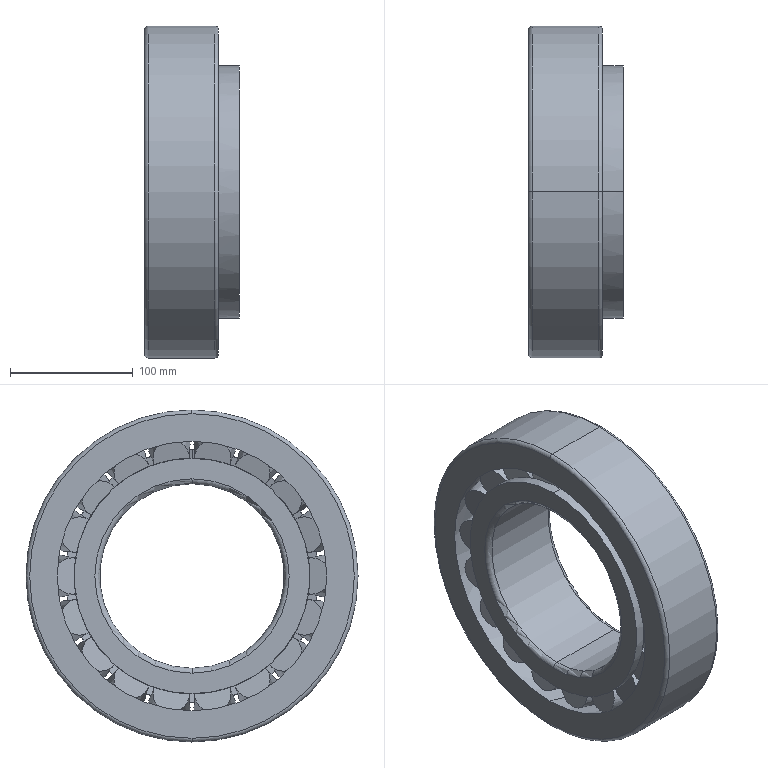Part | NX | features BREP 1 | 1 solid | 151 faces | box 77 x 270 x 270 mm | volume 2111667 mm3 | cone 95 | plane 40 | torus 8 | cylinder 8 | commonest cylinder face diameters 150 x2 191.494 x2 205.326 x2 270 x2